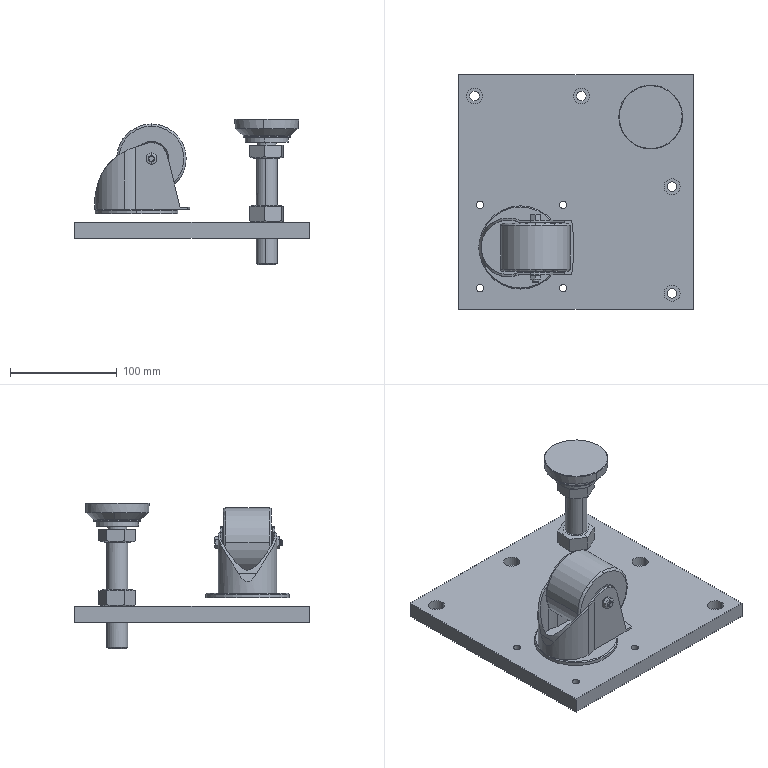Part | SolidWorks | 9 solids | 222 faces | box 220 x 220 x 136.5 mm | volume 999852 mm3 | plane 78 | cylinder 76 | cone 38 | torus 26 | sphere 4 | commonest cylinder face diameters 6.8 x8 9 x8 15 x8 7 x4 8 x4 20 x4